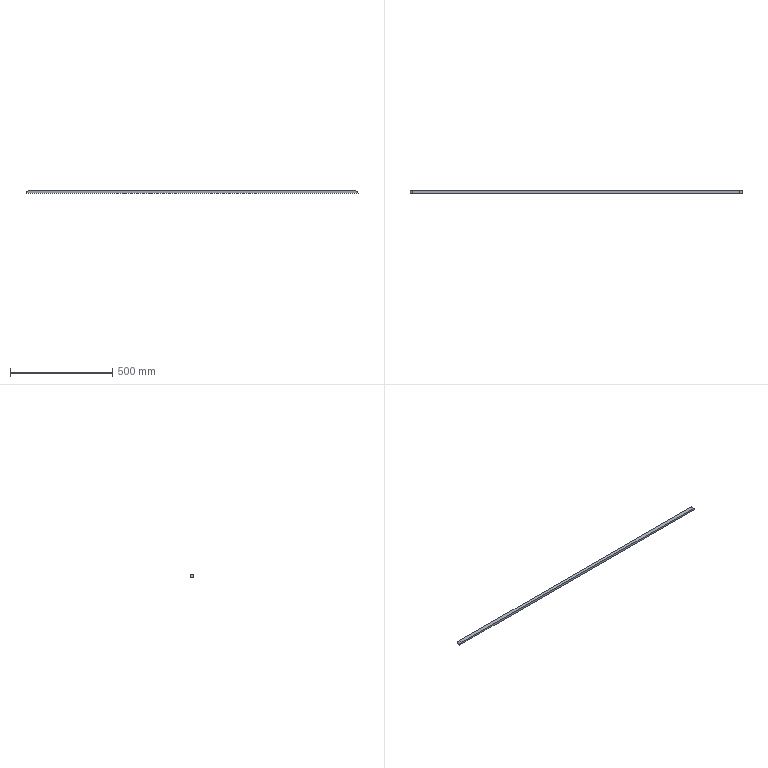Part | STEP file | 1 solid | 6 faces | box 1620 x 17.6 x 10 mm | volume 284365 mm3 | plane 4 | cylinder 2 | commonest cylinder face diameters 20 x2
STEP:
#1=CARTESIAN_POINT('',(0.,0.,0.));
#2=DIRECTION('',(0.,0.,1.));
#3=DIRECTION('',(1.,0.,0.));
#4=AXIS2_PLACEMENT_3D('',#1,#2,#3);
#5=CARTESIAN_POINT('',(1620.,0.,0.));
#6=VERTEX_POINT('',#5);
#7=CARTESIAN_POINT('',(1620.,17.6,0.));
#8=VERTEX_POINT('',#7);
#9=CARTESIAN_POINT('',(1620.,0.,0.));
#10=DIRECTION('',(0.,1.,0.));
#11=VECTOR('',#10,1.);
#12=LINE('',#9,#11);
#13=CARTESIAN_POINT('',(0.,0.,0.));
#14=DIRECTION('',(0.,0.,1.));
#15=DIRECTION('',(1.,0.,0.));
#16=AXIS2_PLACEMENT_3D('',#13,#14,#15);
#17=PLANE('',#16);
#18=CARTESIAN_POINT('',(1620.,0.));
#19=DIRECTION('',(0.,1.));
#20=VECTOR('',#19,1.);
#21=LINE('',#18,#20);
#22=(GEOMETRIC_REPRESENTATION_CONTEXT(2)PARAMETRIC_REPRESENTATION_CONTEXT()REPRESENTATION_CONTEXT('',''));
#23=DEFINITIONAL_REPRESENTATION('',(#21),#22);
#24=PCURVE('',#17,#23);
#25=CARTESIAN_POINT('',(1610.,0.,0.));
#26=DIRECTION('',(0.,1.,0.));
#27=DIRECTION('',(0.,0.,1.));
#28=AXIS2_PLACEMENT_3D('',#25,#26,#27);
#29=CYLINDRICAL_SURFACE('',#28,10.);
#30=CARTESIAN_POINT('',(1.571,0.));
#31=DIRECTION('',(0.,1.));
#32=VECTOR('',#31,1.);
#33=LINE('',#30,#32);
#34=(GEOMETRIC_REPRESENTATION_CONTEXT(2)PARAMETRIC_REPRESENTATION_CONTEXT()REPRESENTATION_CONTEXT('',''));
#35=DEFINITIONAL_REPRESENTATION('',(#33),#34);
#36=PCURVE('',#29,#35);
#37=SURFACE_CURVE('',#12,(#24,#36),.PCURVE_S1.);
#38=EDGE_CURVE('',#6,#8,#37,.T.);
#39=ORIENTED_EDGE('',*,*,#38,.F.);
#40=CARTESIAN_POINT('',(0.,0.,0.));
#41=VERTEX_POINT('',#40);
#42=CARTESIAN_POINT('',(0.,0.,0.));
#43=DIRECTION('',(1.,0.,0.));
#44=VECTOR('',#43,1.);
#45=LINE('',#42,#44);
#46=CARTESIAN_POINT('',(0.,0.));
#47=DIRECTION('',(1.,0.));
#48=VECTOR('',#47,1.);
#49=LINE('',#46,#48);
#50=(GEOMETRIC_REPRESENTATION_CONTEXT(2)PARAMETRIC_REPRESENTATION_CONTEXT()REPRESENTATION_CONTEXT('',''));
#51=DEFINITIONAL_REPRESENTATION('',(#49),#50);
#52=PCURVE('',#17,#51);
#53=CARTESIAN_POINT('',(0.,0.,10.));
#54=DIRECTION('',(0.,1.,0.));
#55=DIRECTION('',(0.,0.,1.));
#56=AXIS2_PLACEMENT_3D('',#53,#54,#55);
#57=PLANE('',#56);
#58=CARTESIAN_POINT('',(-10.,0.));
#59=DIRECTION('',(0.,1.));
#60=VECTOR('',#59,1.);
#61=LINE('',#58,#60);
#62=(GEOMETRIC_REPRESENTATION_CONTEXT(2)PARAMETRIC_REPRESENTATION_CONTEXT()REPRESENTATION_CONTEXT('',''));
#63=DEFINITIONAL_REPRESENTATION('',(#61),#62);
#64=PCURVE('',#57,#63);
#65=SURFACE_CURVE('',#45,(#52,#64),.PCURVE_S1.);
#66=EDGE_CURVE('',#41,#6,#65,.T.);
#67=ORIENTED_EDGE('',*,*,#66,.F.);
#68=CARTESIAN_POINT('',(0.,17.6,0.));
#69=VERTEX_POINT('',#68);
#70=CARTESIAN_POINT('',(0.,0.,0.));
#71=DIRECTION('',(0.,-1.,0.));
#72=VECTOR('',#71,1.);
#73=LINE('',#70,#72);
#74=CARTESIAN_POINT('',(0.,0.));
#75=DIRECTION('',(0.,-1.));
#76=VECTOR('',#75,1.);
#77=LINE('',#74,#76);
#78=(GEOMETRIC_REPRESENTATION_CONTEXT(2)PARAMETRIC_REPRESENTATION_CONTEXT()REPRESENTATION_CONTEXT('',''));
#79=DEFINITIONAL_REPRESENTATION('',(#77),#78);
#80=PCURVE('',#17,#79);
#81=CARTESIAN_POINT('',(10.,0.,0.));
#82=DIRECTION('',(0.,-1.,0.));
#83=DIRECTION('',(0.,0.,-1.));
#84=AXIS2_PLACEMENT_3D('',#81,#82,#83);
#85=CYLINDRICAL_SURFACE('',#84,10.);
#86=CARTESIAN_POINT('',(4.712,0.));
#87=DIRECTION('',(0.,1.));
#88=VECTOR('',#87,1.);
#89=LINE('',#86,#88);
#90=(GEOMETRIC_REPRESENTATION_CONTEXT(2)PARAMETRIC_REPRESENTATION_CONTEXT()REPRESENTATION_CONTEXT('',''));
#91=DEFINITIONAL_REPRESENTATION('',(#89),#90);
#92=PCURVE('',#85,#91);
#93=SURFACE_CURVE('',#73,(#80,#92),.PCURVE_S1.);
#94=EDGE_CURVE('',#69,#41,#93,.T.);
#95=ORIENTED_EDGE('',*,*,#94,.F.);
#96=CARTESIAN_POINT('',(0.,17.6,0.));
#97=DIRECTION('',(-1.,0.,0.));
#98=VECTOR('',#97,1.);
#99=LINE('',#96,#98);
#100=CARTESIAN_POINT('',(0.,17.6));
#101=DIRECTION('',(-1.,0.));
#102=VECTOR('',#101,1.);
#103=LINE('',#100,#102);
#104=(GEOMETRIC_REPRESENTATION_CONTEXT(2)PARAMETRIC_REPRESENTATION_CONTEXT()REPRESENTATION_CONTEXT('',''));
#105=DEFINITIONAL_REPRESENTATION('',(#103),#104);
#106=PCURVE('',#17,#105);
#107=CARTESIAN_POINT('',(0.,17.6,10.));
#108=DIRECTION('',(0.,-1.,0.));
#109=DIRECTION('',(0.,0.,-1.));
#110=AXIS2_PLACEMENT_3D('',#107,#108,#109);
#111=PLANE('',#110);
#112=CARTESIAN_POINT('',(10.,0.));
#113=DIRECTION('',(0.,-1.));
#114=VECTOR('',#113,1.);
#115=LINE('',#112,#114);
#116=(GEOMETRIC_REPRESENTATION_CONTEXT(2)PARAMETRIC_REPRESENTATION_CONTEXT()REPRESENTATION_CONTEXT('',''));
#117=DEFINITIONAL_REPRESENTATION('',(#115),#116);
#118=PCURVE('',#111,#117);
#119=SURFACE_CURVE('',#99,(#106,#118),.PCURVE_S1.);
#120=EDGE_CURVE('',#8,#69,#119,.T.);
#121=ORIENTED_EDGE('',*,*,#120,.F.);
#122=EDGE_LOOP('',(#39,#67,#95,#121));
#123=FACE_BOUND('',#122,.T.);
#124=ADVANCED_FACE('',(#123),#17,.F.);
#125=ORIENTED_EDGE('',*,*,#120,.T.);
#126=CARTESIAN_POINT('',(10.,17.6,10.));
#127=VERTEX_POINT('',#126);
#128=CARTESIAN_POINT('',(10.,17.6,0.));
#129=DIRECTION('',(0.,-1.,0.));
#130=DIRECTION('',(0.,0.,-1.));
#131=AXIS2_PLACEMENT_3D('',#128,#129,#130);
#132=CIRCLE('',#131,10.);
#133=CARTESIAN_POINT('',(10.,10.));
#134=DIRECTION('',(1.,0.));
#135=AXIS2_PLACEMENT_2D('',#133,#134);
#136=CIRCLE('',#135,10.);
#137=(GEOMETRIC_REPRESENTATION_CONTEXT(2)PARAMETRIC_REPRESENTATION_CONTEXT()REPRESENTATION_CONTEXT('',''));
#138=DEFINITIONAL_REPRESENTATION('',(#136),#137);
#139=PCURVE('',#111,#138);
#140=CARTESIAN_POINT('',(0.,-17.6));
#141=DIRECTION('',(1.,0.));
#142=VECTOR('',#141,1.);
#143=LINE('',#140,#142);
#144=(GEOMETRIC_REPRESENTATION_CONTEXT(2)PARAMETRIC_REPRESENTATION_CONTEXT()REPRESENTATION_CONTEXT('',''));
#145=DEFINITIONAL_REPRESENTATION('',(#143),#144);
#146=PCURVE('',#85,#145);
#147=SURFACE_CURVE('',#132,(#139,#146),.PCURVE_S1.);
#148=EDGE_CURVE('',#127,#69,#147,.T.);
#149=ORIENTED_EDGE('',*,*,#148,.F.);
#150=CARTESIAN_POINT('',(1610.,17.6,10.));
#151=VERTEX_POINT('',#150);
#152=CARTESIAN_POINT('',(0.,17.6,10.));
#153=DIRECTION('',(-1.,0.,0.));
#154=VECTOR('',#153,1.);
#155=LINE('',#152,#154);
#156=CARTESIAN_POINT('',(0.,0.));
#157=DIRECTION('',(0.,-1.));
#158=VECTOR('',#157,1.);
#159=LINE('',#156,#158);
#160=(GEOMETRIC_REPRESENTATION_CONTEXT(2)PARAMETRIC_REPRESENTATION_CONTEXT()REPRESENTATION_CONTEXT('',''));
#161=DEFINITIONAL_REPRESENTATION('',(#159),#160);
#162=PCURVE('',#111,#161);
#163=CARTESIAN_POINT('',(0.,0.,10.));
#164=DIRECTION('',(0.,0.,1.));
#165=DIRECTION('',(1.,0.,0.));
#166=AXIS2_PLACEMENT_3D('',#163,#164,#165);
#167=PLANE('',#166);
#168=CARTESIAN_POINT('',(0.,17.6));
#169=DIRECTION('',(-1.,0.));
#170=VECTOR('',#169,1.);
#171=LINE('',#168,#170);
#172=(GEOMETRIC_REPRESENTATION_CONTEXT(2)PARAMETRIC_REPRESENTATION_CONTEXT()REPRESENTATION_CONTEXT('',''));
#173=DEFINITIONAL_REPRESENTATION('',(#171),#172);
#174=PCURVE('',#167,#173);
#175=SURFACE_CURVE('',#155,(#162,#174),.PCURVE_S1.);
#176=EDGE_CURVE('',#151,#127,#175,.T.);
#177=ORIENTED_EDGE('',*,*,#176,.F.);
#178=CARTESIAN_POINT('',(1610.,17.6,0.));
#179=DIRECTION('',(0.,-1.,0.));
#180=DIRECTION('',(0.,0.,1.));
#181=AXIS2_PLACEMENT_3D('',#178,#179,#180);
#182=CIRCLE('',#181,10.);
#183=CARTESIAN_POINT('',(10.,1610.));
#184=DIRECTION('',(-1.,0.));
#185=AXIS2_PLACEMENT_2D('',#183,#184);
#186=CIRCLE('',#185,10.);
#187=(GEOMETRIC_REPRESENTATION_CONTEXT(2)PARAMETRIC_REPRESENTATION_CONTEXT()REPRESENTATION_CONTEXT('',''));
#188=DEFINITIONAL_REPRESENTATION('',(#186),#187);
#189=PCURVE('',#111,#188);
#190=CARTESIAN_POINT('',(6.283,17.6));
#191=DIRECTION('',(-1.,0.));
#192=VECTOR('',#191,1.);
#193=LINE('',#190,#192);
#194=(GEOMETRIC_REPRESENTATION_CONTEXT(2)PARAMETRIC_REPRESENTATION_CONTEXT()REPRESENTATION_CONTEXT('',''));
#195=DEFINITIONAL_REPRESENTATION('',(#193),#194);
#196=PCURVE('',#29,#195);
#197=SURFACE_CURVE('',#182,(#189,#196),.PCURVE_S1.);
#198=EDGE_CURVE('',#8,#151,#197,.T.);
#199=ORIENTED_EDGE('',*,*,#198,.F.);
#200=EDGE_LOOP('',(#125,#149,#177,#199));
#201=FACE_BOUND('',#200,.T.);
#202=ADVANCED_FACE('',(#201),#111,.F.);
#203=CARTESIAN_POINT('',(1610.,0.,10.));
#204=VERTEX_POINT('',#203);
#205=CARTESIAN_POINT('',(1610.,0.,0.));
#206=DIRECTION('',(0.,1.,0.));
#207=DIRECTION('',(0.,0.,1.));
#208=AXIS2_PLACEMENT_3D('',#205,#206,#207);
#209=CIRCLE('',#208,10.);
#210=CARTESIAN_POINT('',(0.,0.));
#211=DIRECTION('',(1.,0.));
#212=VECTOR('',#211,1.);
#213=LINE('',#210,#212);
#214=(GEOMETRIC_REPRESENTATION_CONTEXT(2)PARAMETRIC_REPRESENTATION_CONTEXT()REPRESENTATION_CONTEXT('',''));
#215=DEFINITIONAL_REPRESENTATION('',(#213),#214);
#216=PCURVE('',#29,#215);
#217=CARTESIAN_POINT('',(-10.,1610.));
#218=DIRECTION('',(1.,0.));
#219=AXIS2_PLACEMENT_2D('',#217,#218);
#220=CIRCLE('',#219,10.);
#221=(GEOMETRIC_REPRESENTATION_CONTEXT(2)PARAMETRIC_REPRESENTATION_CONTEXT()REPRESENTATION_CONTEXT('',''));
#222=DEFINITIONAL_REPRESENTATION('',(#220),#221);
#223=PCURVE('',#57,#222);
#224=SURFACE_CURVE('',#209,(#216,#223),.PCURVE_S1.);
#225=EDGE_CURVE('',#204,#6,#224,.T.);
#226=ORIENTED_EDGE('',*,*,#225,.T.);
#227=ORIENTED_EDGE('',*,*,#38,.T.);
#228=ORIENTED_EDGE('',*,*,#198,.T.);
#229=CARTESIAN_POINT('',(1610.,0.,10.));
#230=DIRECTION('',(0.,-1.,0.));
#231=VECTOR('',#230,1.);
#232=LINE('',#229,#231);
#233=CARTESIAN_POINT('',(0.,0.));
#234=DIRECTION('',(0.,-1.));
#235=VECTOR('',#234,1.);
#236=LINE('',#233,#235);
#237=(GEOMETRIC_REPRESENTATION_CONTEXT(2)PARAMETRIC_REPRESENTATION_CONTEXT()REPRESENTATION_CONTEXT('',''));
#238=DEFINITIONAL_REPRESENTATION('',(#236),#237);
#239=PCURVE('',#29,#238);
#240=CARTESIAN_POINT('',(1610.,0.));
#241=DIRECTION('',(0.,-1.));
#242=VECTOR('',#241,1.);
#243=LINE('',#240,#242);
#244=(GEOMETRIC_REPRESENTATION_CONTEXT(2)PARAMETRIC_REPRESENTATION_CONTEXT()REPRESENTATION_CONTEXT('',''));
#245=DEFINITIONAL_REPRESENTATION('',(#243),#244);
#246=PCURVE('',#167,#245);
#247=SURFACE_CURVE('',#232,(#239,#246),.PCURVE_S1.);
#248=EDGE_CURVE('',#151,#204,#247,.T.);
#249=ORIENTED_EDGE('',*,*,#248,.T.);
#250=EDGE_LOOP('',(#226,#227,#228,#249));
#251=FACE_BOUND('',#250,.T.);
#252=ADVANCED_FACE('',(#251),#29,.T.);
#253=CARTESIAN_POINT('',(10.,0.,10.));
#254=VERTEX_POINT('',#253);
#255=CARTESIAN_POINT('',(0.,0.,10.));
#256=DIRECTION('',(1.,0.,0.));
#257=VECTOR('',#256,1.);
#258=LINE('',#255,#257);
#259=CARTESIAN_POINT('',(0.,0.));
#260=DIRECTION('',(0.,1.));
#261=VECTOR('',#260,1.);
#262=LINE('',#259,#261);
#263=(GEOMETRIC_REPRESENTATION_CONTEXT(2)PARAMETRIC_REPRESENTATION_CONTEXT()REPRESENTATION_CONTEXT('',''));
#264=DEFINITIONAL_REPRESENTATION('',(#262),#263);
#265=PCURVE('',#57,#264);
#266=CARTESIAN_POINT('',(0.,0.));
#267=DIRECTION('',(1.,0.));
#268=VECTOR('',#267,1.);
#269=LINE('',#266,#268);
#270=(GEOMETRIC_REPRESENTATION_CONTEXT(2)PARAMETRIC_REPRESENTATION_CONTEXT()REPRESENTATION_CONTEXT('',''));
#271=DEFINITIONAL_REPRESENTATION('',(#269),#270);
#272=PCURVE('',#167,#271);
#273=SURFACE_CURVE('',#258,(#265,#272),.PCURVE_S1.);
#274=EDGE_CURVE('',#254,#204,#273,.T.);
#275=ORIENTED_EDGE('',*,*,#274,.F.);
#276=CARTESIAN_POINT('',(10.,0.,0.));
#277=DIRECTION('',(0.,1.,0.));
#278=DIRECTION('',(0.,0.,-1.));
#279=AXIS2_PLACEMENT_3D('',#276,#277,#278);
#280=CIRCLE('',#279,10.);
#281=CARTESIAN_POINT('',(-10.,10.));
#282=DIRECTION('',(-1.,0.));
#283=AXIS2_PLACEMENT_2D('',#281,#282);
#284=CIRCLE('',#283,10.);
#285=(GEOMETRIC_REPRESENTATION_CONTEXT(2)PARAMETRIC_REPRESENTATION_CONTEXT()REPRESENTATION_CONTEXT('',''));
#286=DEFINITIONAL_REPRESENTATION('',(#284),#285);
#287=PCURVE('',#57,#286);
#288=CARTESIAN_POINT('',(6.283,0.));
#289=DIRECTION('',(-1.,0.));
#290=VECTOR('',#289,1.);
#291=LINE('',#288,#290);
#292=(GEOMETRIC_REPRESENTATION_CONTEXT(2)PARAMETRIC_REPRESENTATION_CONTEXT()REPRESENTATION_CONTEXT('',''));
#293=DEFINITIONAL_REPRESENTATION('',(#291),#292);
#294=PCURVE('',#85,#293);
#295=SURFACE_CURVE('',#280,(#287,#294),.PCURVE_S1.);
#296=EDGE_CURVE('',#41,#254,#295,.T.);
#297=ORIENTED_EDGE('',*,*,#296,.F.);
#298=ORIENTED_EDGE('',*,*,#66,.T.);
#299=ORIENTED_EDGE('',*,*,#225,.F.);
#300=EDGE_LOOP('',(#275,#297,#298,#299));
#301=FACE_BOUND('',#300,.T.);
#302=ADVANCED_FACE('',(#301),#57,.F.);
#303=ORIENTED_EDGE('',*,*,#148,.T.);
#304=ORIENTED_EDGE('',*,*,#94,.T.);
#305=ORIENTED_EDGE('',*,*,#296,.T.);
#306=CARTESIAN_POINT('',(10.,0.,10.));
#307=DIRECTION('',(0.,1.,0.));
#308=VECTOR('',#307,1.);
#309=LINE('',#306,#308);
#310=CARTESIAN_POINT('',(3.142,0.));
#311=DIRECTION('',(0.,-1.));
#312=VECTOR('',#311,1.);
#313=LINE('',#310,#312);
#314=(GEOMETRIC_REPRESENTATION_CONTEXT(2)PARAMETRIC_REPRESENTATION_CONTEXT()REPRESENTATION_CONTEXT('',''));
#315=DEFINITIONAL_REPRESENTATION('',(#313),#314);
#316=PCURVE('',#85,#315);
#317=CARTESIAN_POINT('',(10.,0.));
#318=DIRECTION('',(0.,1.));
#319=VECTOR('',#318,1.);
#320=LINE('',#317,#319);
#321=(GEOMETRIC_REPRESENTATION_CONTEXT(2)PARAMETRIC_REPRESENTATION_CONTEXT()REPRESENTATION_CONTEXT('',''));
#322=DEFINITIONAL_REPRESENTATION('',(#320),#321);
#323=PCURVE('',#167,#322);
#324=SURFACE_CURVE('',#309,(#316,#323),.PCURVE_S1.);
#325=EDGE_CURVE('',#254,#127,#324,.T.);
#326=ORIENTED_EDGE('',*,*,#325,.T.);
#327=EDGE_LOOP('',(#303,#304,#305,#326));
#328=FACE_BOUND('',#327,.T.);
#329=ADVANCED_FACE('',(#328),#85,.T.);
#330=ORIENTED_EDGE('',*,*,#274,.T.);
#331=ORIENTED_EDGE('',*,*,#248,.F.);
#332=ORIENTED_EDGE('',*,*,#176,.T.);
#333=ORIENTED_EDGE('',*,*,#325,.F.);
#334=EDGE_LOOP('',(#330,#331,#332,#333));
#335=FACE_BOUND('',#334,.T.);
#336=ADVANCED_FACE('',(#335),#167,.T.);
#337=CLOSED_SHELL('',(#124,#202,#252,#302,#329,#336));
#338=MANIFOLD_SOLID_BREP('',#337);
#339=(LENGTH_UNIT()NAMED_UNIT(*)SI_UNIT(.MILLI.,.METRE.));
#340=UNCERTAINTY_MEASURE_WITH_UNIT(LENGTH_MEASURE(0.0000001),#339,'','');
#341=(NAMED_UNIT(*)PLANE_ANGLE_UNIT()SI_UNIT($,.RADIAN.));
#342=(NAMED_UNIT(*)SI_UNIT($,.STERADIAN.)SOLID_ANGLE_UNIT());
#343=(GEOMETRIC_REPRESENTATION_CONTEXT(3)GLOBAL_UNCERTAINTY_ASSIGNED_CONTEXT((#340))GLOBAL_UNIT_ASSIGNED_CONTEXT((#339,#341,#342))REPRESENTATION_CONTEXT('',''));
#344=ADVANCED_BREP_SHAPE_REPRESENTATION('',(#4,#338),#343);